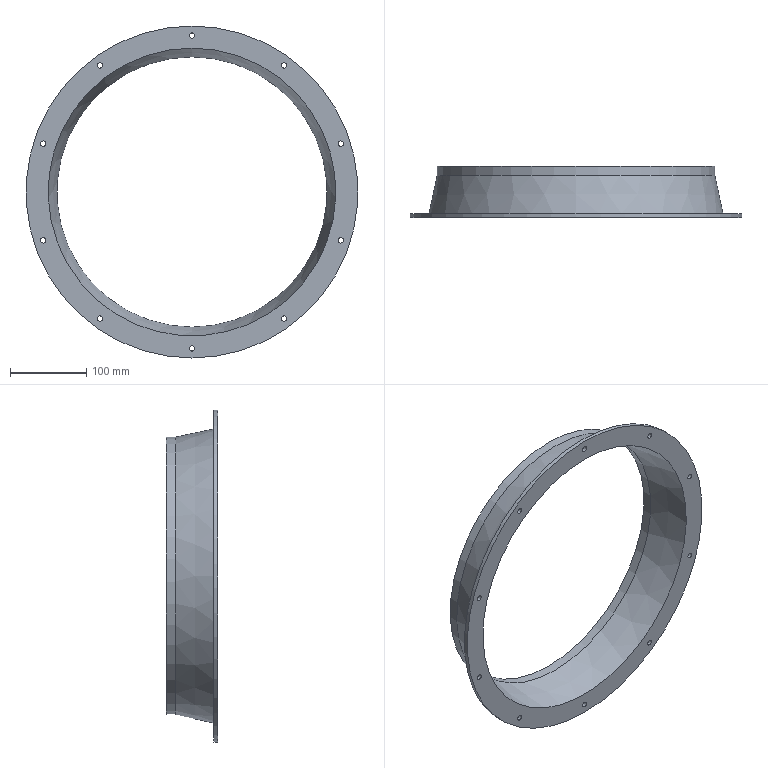Part | STEP file | Upper cover | 1 solid | 18 faces | box 435 x 67 x 435 mm | volume 550559 mm3 | cylinder 13 | plane 3 | cone 2 | commonest cylinder face diameters 7 x10 354 x1 364 x1 435 x1
STEP:
#1=CARTESIAN_POINT('',(0.,67.,182.));
#2=VERTEX_POINT('',#1);
#3=CARTESIAN_POINT('',(0.,67.,0.));
#4=DIRECTION('',(0.,1.,0.));
#5=DIRECTION('',(0.,0.,1.));
#6=AXIS2_PLACEMENT_3D('',#3,#4,#5);
#7=CIRCLE('',#6,182.);
#8=EDGE_CURVE('',#2,#2,#7,.F.);
#9=ORIENTED_EDGE('',*,*,#8,.T.);
#10=EDGE_LOOP('',(#9));
#11=FACE_OUTER_BOUND('',#10,.T.);
#12=CARTESIAN_POINT('',(0.,55.,182.));
#13=VERTEX_POINT('',#12);
#14=CARTESIAN_POINT('',(0.,55.,0.));
#15=DIRECTION('',(0.,1.,0.));
#16=DIRECTION('',(0.,0.,1.));
#17=AXIS2_PLACEMENT_3D('',#14,#15,#16);
#18=CIRCLE('',#17,182.);
#19=EDGE_CURVE('',#13,#13,#18,.T.);
#20=ORIENTED_EDGE('',*,*,#19,.T.);
#21=EDGE_LOOP('',(#20));
#22=FACE_OUTER_BOUND('',#21,.T.);
#23=CARTESIAN_POINT('',(0.,55.,0.));
#24=DIRECTION('',(0.,1.,0.));
#25=DIRECTION('',(0.,0.,1.));
#26=AXIS2_PLACEMENT_3D('',#23,#24,#25);
#27=CYLINDRICAL_SURFACE('',#26,182.);
#28=ADVANCED_FACE('',(#11,#22),#27,.T.);
#29=CARTESIAN_POINT('',(0.,67.,177.));
#30=VERTEX_POINT('',#29);
#31=CARTESIAN_POINT('',(0.,67.,0.));
#32=DIRECTION('',(0.,1.,0.));
#33=DIRECTION('',(0.,0.,1.));
#34=AXIS2_PLACEMENT_3D('',#31,#32,#33);
#35=CIRCLE('',#34,177.);
#36=EDGE_CURVE('',#30,#30,#35,.T.);
#37=ORIENTED_EDGE('',*,*,#36,.T.);
#38=EDGE_LOOP('',(#37));
#39=FACE_OUTER_BOUND('',#38,.T.);
#40=CARTESIAN_POINT('',(0.,54.481,177.));
#41=VERTEX_POINT('',#40);
#42=CARTESIAN_POINT('',(0.,54.481,0.));
#43=DIRECTION('',(0.,1.,0.));
#44=DIRECTION('',(0.,0.,1.));
#45=AXIS2_PLACEMENT_3D('',#42,#43,#44);
#46=CIRCLE('',#45,177.);
#47=EDGE_CURVE('',#41,#41,#46,.T.);
#48=ORIENTED_EDGE('',*,*,#47,.F.);
#49=EDGE_LOOP('',(#48));
#50=FACE_OUTER_BOUND('',#49,.T.);
#51=CARTESIAN_POINT('',(0.,85.,0.));
#52=DIRECTION('',(0.,1.,0.));
#53=DIRECTION('',(0.,0.,1.));
#54=AXIS2_PLACEMENT_3D('',#51,#52,#53);
#55=CYLINDRICAL_SURFACE('',#54,177.);
#56=ADVANCED_FACE('',(#39,#50),#55,.F.);
#57=ORIENTED_EDGE('',*,*,#8,.F.);
#58=EDGE_LOOP('',(#57));
#59=FACE_BOUND('',#58,.T.);
#60=ORIENTED_EDGE('',*,*,#36,.F.);
#61=EDGE_LOOP('',(#60));
#62=FACE_BOUND('',#61,.T.);
#63=CARTESIAN_POINT('',(0.,67.,182.));
#64=DIRECTION('',(0.,1.,0.));
#65=DIRECTION('',(1.,0.,0.));
#66=AXIS2_PLACEMENT_3D('',#63,#64,#65);
#67=PLANE('',#66);
#68=ADVANCED_FACE('',(#59,#62),#67,.T.);
#69=ORIENTED_EDGE('',*,*,#19,.F.);
#70=EDGE_LOOP('',(#69));
#71=FACE_OUTER_BOUND('',#70,.T.);
#72=CARTESIAN_POINT('',(0.,5.,192.5));
#73=VERTEX_POINT('',#72);
#74=CARTESIAN_POINT('',(0.,5.,0.));
#75=DIRECTION('',(0.,1.,0.));
#76=DIRECTION('',(0.,0.,1.));
#77=AXIS2_PLACEMENT_3D('',#74,#75,#76);
#78=CIRCLE('',#77,192.5);
#79=EDGE_CURVE('',#73,#73,#78,.T.);
#80=ORIENTED_EDGE('',*,*,#79,.T.);
#81=EDGE_LOOP('',(#80));
#82=FACE_OUTER_BOUND('',#81,.T.);
#83=CARTESIAN_POINT('',(0.,30.,0.));
#84=DIRECTION('',(0.,-1.,0.));
#85=DIRECTION('',(0.,0.,-1.));
#86=AXIS2_PLACEMENT_3D('',#83,#84,#85);
#87=CONICAL_SURFACE('',#86,187.25,0.207);
#88=ADVANCED_FACE('',(#71,#82),#87,.T.);
#89=ORIENTED_EDGE('',*,*,#47,.T.);
#90=EDGE_LOOP('',(#89));
#91=FACE_OUTER_BOUND('',#90,.T.);
#92=CARTESIAN_POINT('',(0.,0.,188.441));
#93=VERTEX_POINT('',#92);
#94=CARTESIAN_POINT('',(0.,0.,0.));
#95=DIRECTION('',(0.,1.,0.));
#96=DIRECTION('',(0.,0.,1.));
#97=AXIS2_PLACEMENT_3D('',#94,#95,#96);
#98=CIRCLE('',#97,188.441);
#99=EDGE_CURVE('',#93,#93,#98,.T.);
#100=ORIENTED_EDGE('',*,*,#99,.F.);
#101=EDGE_LOOP('',(#100));
#102=FACE_OUTER_BOUND('',#101,.T.);
#103=CARTESIAN_POINT('',(0.,27.24,0.));
#104=DIRECTION('',(0.,-1.,0.));
#105=DIRECTION('',(0.,0.,-1.));
#106=AXIS2_PLACEMENT_3D('',#103,#104,#105);
#107=CONICAL_SURFACE('',#106,182.72,0.207);
#108=ADVANCED_FACE('',(#91,#102),#107,.F.);
#109=CARTESIAN_POINT('',(0.,5.,217.5));
#110=VERTEX_POINT('',#109);
#111=CARTESIAN_POINT('',(0.,5.,0.));
#112=DIRECTION('',(0.,1.,0.));
#113=DIRECTION('',(0.,0.,1.));
#114=AXIS2_PLACEMENT_3D('',#111,#112,#113);
#115=CIRCLE('',#114,217.5);
#116=EDGE_CURVE('',#110,#110,#115,.T.);
#117=ORIENTED_EDGE('',*,*,#116,.T.);
#118=EDGE_LOOP('',(#117));
#119=FACE_BOUND('',#118,.T.);
#120=CARTESIAN_POINT('',(123.328,5.,163.791));
#121=VERTEX_POINT('',#120);
#122=CARTESIAN_POINT('',(120.496,5.,165.848));
#123=DIRECTION('',(0.,1.,0.));
#124=DIRECTION('',(0.809,0.,-0.5878));
#125=AXIS2_PLACEMENT_3D('',#122,#123,#124);
#126=CIRCLE('',#125,3.5);
#127=EDGE_CURVE('',#121,#121,#126,.F.);
#128=ORIENTED_EDGE('',*,*,#127,.T.);
#129=EDGE_LOOP('',(#128));
#130=FACE_BOUND('',#129,.T.);
#131=CARTESIAN_POINT('',(196.048,5.,60.02));
#132=VERTEX_POINT('',#131);
#133=CARTESIAN_POINT('',(194.967,5.,63.348));
#134=DIRECTION('',(0.,1.,0.));
#135=DIRECTION('',(0.309,0.,-0.9511));
#136=AXIS2_PLACEMENT_3D('',#133,#134,#135);
#137=CIRCLE('',#136,3.5);
#138=EDGE_CURVE('',#132,#132,#137,.F.);
#139=ORIENTED_EDGE('',*,*,#138,.T.);
#140=EDGE_LOOP('',(#139));
#141=FACE_BOUND('',#140,.T.);
#142=CARTESIAN_POINT('',(193.885,5.,-66.677));
#143=VERTEX_POINT('',#142);
#144=CARTESIAN_POINT('',(194.967,5.,-63.348));
#145=DIRECTION('',(0.,1.,0.));
#146=DIRECTION('',(-0.309,0.,-0.9511));
#147=AXIS2_PLACEMENT_3D('',#144,#145,#146);
#148=CIRCLE('',#147,3.5);
#149=EDGE_CURVE('',#143,#143,#148,.F.);
#150=ORIENTED_EDGE('',*,*,#149,.T.);
#151=EDGE_LOOP('',(#150));
#152=FACE_BOUND('',#151,.T.);
#153=CARTESIAN_POINT('',(117.664,5.,-167.906));
#154=VERTEX_POINT('',#153);
#155=CARTESIAN_POINT('',(120.496,5.,-165.848));
#156=DIRECTION('',(0.,1.,0.));
#157=DIRECTION('',(-0.809,0.,-0.5878));
#158=AXIS2_PLACEMENT_3D('',#155,#156,#157);
#159=CIRCLE('',#158,3.5);
#160=EDGE_CURVE('',#154,#154,#159,.F.);
#161=ORIENTED_EDGE('',*,*,#160,.T.);
#162=EDGE_LOOP('',(#161));
#163=FACE_BOUND('',#162,.T.);
#164=CARTESIAN_POINT('',(-3.5,5.,-205.));
#165=VERTEX_POINT('',#164);
#166=CARTESIAN_POINT('',(0.,5.,-205.));
#167=DIRECTION('',(0.,1.,0.));
#168=DIRECTION('',(-1.,0.,0.));
#169=AXIS2_PLACEMENT_3D('',#166,#167,#168);
#170=CIRCLE('',#169,3.5);
#171=EDGE_CURVE('',#165,#165,#170,.F.);
#172=ORIENTED_EDGE('',*,*,#171,.T.);
#173=EDGE_LOOP('',(#172));
#174=FACE_BOUND('',#173,.T.);
#175=CARTESIAN_POINT('',(-123.328,5.,-163.791));
#176=VERTEX_POINT('',#175);
#177=CARTESIAN_POINT('',(-120.496,5.,-165.848));
#178=DIRECTION('',(0.,1.,0.));
#179=DIRECTION('',(-0.809,0.,0.5878));
#180=AXIS2_PLACEMENT_3D('',#177,#178,#179);
#181=CIRCLE('',#180,3.5);
#182=EDGE_CURVE('',#176,#176,#181,.F.);
#183=ORIENTED_EDGE('',*,*,#182,.T.);
#184=EDGE_LOOP('',(#183));
#185=FACE_BOUND('',#184,.T.);
#186=CARTESIAN_POINT('',(-196.048,5.,-60.02));
#187=VERTEX_POINT('',#186);
#188=CARTESIAN_POINT('',(-194.967,5.,-63.348));
#189=DIRECTION('',(0.,1.,0.));
#190=DIRECTION('',(-0.309,0.,0.9511));
#191=AXIS2_PLACEMENT_3D('',#188,#189,#190);
#192=CIRCLE('',#191,3.5);
#193=EDGE_CURVE('',#187,#187,#192,.F.);
#194=ORIENTED_EDGE('',*,*,#193,.T.);
#195=EDGE_LOOP('',(#194));
#196=FACE_BOUND('',#195,.T.);
#197=CARTESIAN_POINT('',(-193.885,5.,66.677));
#198=VERTEX_POINT('',#197);
#199=CARTESIAN_POINT('',(-194.967,5.,63.348));
#200=DIRECTION('',(0.,1.,0.));
#201=DIRECTION('',(0.309,0.,0.9511));
#202=AXIS2_PLACEMENT_3D('',#199,#200,#201);
#203=CIRCLE('',#202,3.5);
#204=EDGE_CURVE('',#198,#198,#203,.F.);
#205=ORIENTED_EDGE('',*,*,#204,.T.);
#206=EDGE_LOOP('',(#205));
#207=FACE_BOUND('',#206,.T.);
#208=CARTESIAN_POINT('',(-117.664,5.,167.906));
#209=VERTEX_POINT('',#208);
#210=CARTESIAN_POINT('',(-120.496,5.,165.848));
#211=DIRECTION('',(0.,1.,0.));
#212=DIRECTION('',(0.809,0.,0.5878));
#213=AXIS2_PLACEMENT_3D('',#210,#211,#212);
#214=CIRCLE('',#213,3.5);
#215=EDGE_CURVE('',#209,#209,#214,.F.);
#216=ORIENTED_EDGE('',*,*,#215,.T.);
#217=EDGE_LOOP('',(#216));
#218=FACE_BOUND('',#217,.T.);
#219=ORIENTED_EDGE('',*,*,#79,.F.);
#220=EDGE_LOOP('',(#219));
#221=FACE_BOUND('',#220,.T.);
#222=CARTESIAN_POINT('',(3.5,5.,205.));
#223=VERTEX_POINT('',#222);
#224=CARTESIAN_POINT('',(0.,5.,205.));
#225=DIRECTION('',(0.,1.,0.));
#226=DIRECTION('',(1.,0.,0.));
#227=AXIS2_PLACEMENT_3D('',#224,#225,#226);
#228=CIRCLE('',#227,3.5);
#229=EDGE_CURVE('',#223,#223,#228,.F.);
#230=ORIENTED_EDGE('',*,*,#229,.T.);
#231=EDGE_LOOP('',(#230));
#232=FACE_BOUND('',#231,.T.);
#233=CARTESIAN_POINT('',(0.,5.,0.));
#234=DIRECTION('',(0.,1.,0.));
#235=DIRECTION('',(0.,0.,1.));
#236=AXIS2_PLACEMENT_3D('',#233,#234,#235);
#237=PLANE('',#236);
#238=ADVANCED_FACE('',(#119,#130,#141,#152,#163,#174,#185,#196,#207,#218,#221,#232),#237,.T.);
#239=CARTESIAN_POINT('',(0.,0.,217.5));
#240=VERTEX_POINT('',#239);
#241=CARTESIAN_POINT('',(0.,0.,0.));
#242=DIRECTION('',(0.,1.,0.));
#243=DIRECTION('',(0.,0.,1.));
#244=AXIS2_PLACEMENT_3D('',#241,#242,#243);
#245=CIRCLE('',#244,217.5);
#246=EDGE_CURVE('',#240,#240,#245,.T.);
#247=ORIENTED_EDGE('',*,*,#246,.F.);
#248=EDGE_LOOP('',(#247));
#249=FACE_BOUND('',#248,.T.);
#250=CARTESIAN_POINT('',(123.328,0.,163.791));
#251=VERTEX_POINT('',#250);
#252=CARTESIAN_POINT('',(120.496,0.,165.848));
#253=DIRECTION('',(0.,1.,0.));
#254=DIRECTION('',(0.809,0.,-0.5878));
#255=AXIS2_PLACEMENT_3D('',#252,#253,#254);
#256=CIRCLE('',#255,3.5);
#257=EDGE_CURVE('',#251,#251,#256,.T.);
#258=ORIENTED_EDGE('',*,*,#257,.T.);
#259=EDGE_LOOP('',(#258));
#260=FACE_BOUND('',#259,.T.);
#261=CARTESIAN_POINT('',(196.048,0.,60.02));
#262=VERTEX_POINT('',#261);
#263=CARTESIAN_POINT('',(194.967,0.,63.348));
#264=DIRECTION('',(0.,1.,0.));
#265=DIRECTION('',(0.309,0.,-0.9511));
#266=AXIS2_PLACEMENT_3D('',#263,#264,#265);
#267=CIRCLE('',#266,3.5);
#268=EDGE_CURVE('',#262,#262,#267,.T.);
#269=ORIENTED_EDGE('',*,*,#268,.T.);
#270=EDGE_LOOP('',(#269));
#271=FACE_BOUND('',#270,.T.);
#272=CARTESIAN_POINT('',(193.885,0.,-66.677));
#273=VERTEX_POINT('',#272);
#274=CARTESIAN_POINT('',(194.967,0.,-63.348));
#275=DIRECTION('',(0.,1.,0.));
#276=DIRECTION('',(-0.309,0.,-0.9511));
#277=AXIS2_PLACEMENT_3D('',#274,#275,#276);
#278=CIRCLE('',#277,3.5);
#279=EDGE_CURVE('',#273,#273,#278,.T.);
#280=ORIENTED_EDGE('',*,*,#279,.T.);
#281=EDGE_LOOP('',(#280));
#282=FACE_BOUND('',#281,.T.);
#283=CARTESIAN_POINT('',(117.664,0.,-167.906));
#284=VERTEX_POINT('',#283);
#285=CARTESIAN_POINT('',(120.496,0.,-165.848));
#286=DIRECTION('',(0.,1.,0.));
#287=DIRECTION('',(-0.809,0.,-0.5878));
#288=AXIS2_PLACEMENT_3D('',#285,#286,#287);
#289=CIRCLE('',#288,3.5);
#290=EDGE_CURVE('',#284,#284,#289,.T.);
#291=ORIENTED_EDGE('',*,*,#290,.T.);
#292=EDGE_LOOP('',(#291));
#293=FACE_BOUND('',#292,.T.);
#294=CARTESIAN_POINT('',(-3.5,0.,-205.));
#295=VERTEX_POINT('',#294);
#296=CARTESIAN_POINT('',(0.,0.,-205.));
#297=DIRECTION('',(0.,1.,0.));
#298=DIRECTION('',(-1.,0.,0.));
#299=AXIS2_PLACEMENT_3D('',#296,#297,#298);
#300=CIRCLE('',#299,3.5);
#301=EDGE_CURVE('',#295,#295,#300,.T.);
#302=ORIENTED_EDGE('',*,*,#301,.T.);
#303=EDGE_LOOP('',(#302));
#304=FACE_BOUND('',#303,.T.);
#305=CARTESIAN_POINT('',(-123.328,0.,-163.791));
#306=VERTEX_POINT('',#305);
#307=CARTESIAN_POINT('',(-120.496,0.,-165.848));
#308=DIRECTION('',(0.,1.,0.));
#309=DIRECTION('',(-0.809,0.,0.5878));
#310=AXIS2_PLACEMENT_3D('',#307,#308,#309);
#311=CIRCLE('',#310,3.5);
#312=EDGE_CURVE('',#306,#306,#311,.T.);
#313=ORIENTED_EDGE('',*,*,#312,.T.);
#314=EDGE_LOOP('',(#313));
#315=FACE_BOUND('',#314,.T.);
#316=CARTESIAN_POINT('',(-196.048,0.,-60.02));
#317=VERTEX_POINT('',#316);
#318=CARTESIAN_POINT('',(-194.967,0.,-63.348));
#319=DIRECTION('',(0.,1.,0.));
#320=DIRECTION('',(-0.309,0.,0.9511));
#321=AXIS2_PLACEMENT_3D('',#318,#319,#320);
#322=CIRCLE('',#321,3.5);
#323=EDGE_CURVE('',#317,#317,#322,.T.);
#324=ORIENTED_EDGE('',*,*,#323,.T.);
#325=EDGE_LOOP('',(#324));
#326=FACE_BOUND('',#325,.T.);
#327=CARTESIAN_POINT('',(-193.885,0.,66.677));
#328=VERTEX_POINT('',#327);
#329=CARTESIAN_POINT('',(-194.967,0.,63.348));
#330=DIRECTION('',(0.,1.,0.));
#331=DIRECTION('',(0.309,0.,0.9511));
#332=AXIS2_PLACEMENT_3D('',#329,#330,#331);
#333=CIRCLE('',#332,3.5);
#334=EDGE_CURVE('',#328,#328,#333,.T.);
#335=ORIENTED_EDGE('',*,*,#334,.T.);
#336=EDGE_LOOP('',(#335));
#337=FACE_BOUND('',#336,.T.);
#338=CARTESIAN_POINT('',(-117.664,0.,167.906));
#339=VERTEX_POINT('',#338);
#340=CARTESIAN_POINT('',(-120.496,0.,165.848));
#341=DIRECTION('',(0.,1.,0.));
#342=DIRECTION('',(0.809,0.,0.5878));
#343=AXIS2_PLACEMENT_3D('',#340,#341,#342);
#344=CIRCLE('',#343,3.5);
#345=EDGE_CURVE('',#339,#339,#344,.T.);
#346=ORIENTED_EDGE('',*,*,#345,.T.);
#347=EDGE_LOOP('',(#346));
#348=FACE_BOUND('',#347,.T.);
#349=ORIENTED_EDGE('',*,*,#99,.T.);
#350=EDGE_LOOP('',(#349));
#351=FACE_BOUND('',#350,.T.);
#352=CARTESIAN_POINT('',(3.5,0.,205.));
#353=VERTEX_POINT('',#352);
#354=CARTESIAN_POINT('',(0.,0.,205.));
#355=DIRECTION('',(0.,1.,0.));
#356=DIRECTION('',(1.,0.,0.));
#357=AXIS2_PLACEMENT_3D('',#354,#355,#356);
#358=CIRCLE('',#357,3.5);
#359=EDGE_CURVE('',#353,#353,#358,.T.);
#360=ORIENTED_EDGE('',*,*,#359,.T.);
#361=EDGE_LOOP('',(#360));
#362=FACE_BOUND('',#361,.T.);
#363=CARTESIAN_POINT('',(0.,0.,0.));
#364=DIRECTION('',(0.,-1.,0.));
#365=DIRECTION('',(0.,0.,1.));
#366=AXIS2_PLACEMENT_3D('',#363,#364,#365);
#367=PLANE('',#366);
#368=ADVANCED_FACE('',(#249,#260,#271,#282,#293,#304,#315,#326,#337,#348,#351,#362),#367,.T.);
#369=ORIENTED_EDGE('',*,*,#116,.F.);
#370=EDGE_LOOP('',(#369));
#371=FACE_OUTER_BOUND('',#370,.T.);
#372=ORIENTED_EDGE('',*,*,#246,.T.);
#373=EDGE_LOOP('',(#372));
#374=FACE_OUTER_BOUND('',#373,.T.);
#375=CARTESIAN_POINT('',(0.,0.,0.));
#376=DIRECTION('',(0.,1.,0.));
#377=DIRECTION('',(0.,0.,1.));
#378=AXIS2_PLACEMENT_3D('',#375,#376,#377);
#379=CYLINDRICAL_SURFACE('',#378,217.5);
#380=ADVANCED_FACE('',(#371,#374),#379,.T.);
#381=ORIENTED_EDGE('',*,*,#127,.F.);
#382=EDGE_LOOP('',(#381));
#383=FACE_OUTER_BOUND('',#382,.T.);
#384=ORIENTED_EDGE('',*,*,#257,.F.);
#385=EDGE_LOOP('',(#384));
#386=FACE_OUTER_BOUND('',#385,.T.);
#387=CARTESIAN_POINT('',(120.496,-35.,165.848));
#388=DIRECTION('',(0.,1.,0.));
#389=DIRECTION('',(0.809,0.,-0.5878));
#390=AXIS2_PLACEMENT_3D('',#387,#388,#389);
#391=CYLINDRICAL_SURFACE('',#390,3.5);
#392=ADVANCED_FACE('',(#383,#386),#391,.F.);
#393=ORIENTED_EDGE('',*,*,#138,.F.);
#394=EDGE_LOOP('',(#393));
#395=FACE_OUTER_BOUND('',#394,.T.);
#396=ORIENTED_EDGE('',*,*,#268,.F.);
#397=EDGE_LOOP('',(#396));
#398=FACE_OUTER_BOUND('',#397,.T.);
#399=CARTESIAN_POINT('',(194.967,-35.,63.348));
#400=DIRECTION('',(0.,1.,0.));
#401=DIRECTION('',(0.309,0.,-0.9511));
#402=AXIS2_PLACEMENT_3D('',#399,#400,#401);
#403=CYLINDRICAL_SURFACE('',#402,3.5);
#404=ADVANCED_FACE('',(#395,#398),#403,.F.);
#405=ORIENTED_EDGE('',*,*,#149,.F.);
#406=EDGE_LOOP('',(#405));
#407=FACE_OUTER_BOUND('',#406,.T.);
#408=ORIENTED_EDGE('',*,*,#279,.F.);
#409=EDGE_LOOP('',(#408));
#410=FACE_OUTER_BOUND('',#409,.T.);
#411=CARTESIAN_POINT('',(194.967,-35.,-63.348));
#412=DIRECTION('',(0.,1.,0.));
#413=DIRECTION('',(-0.309,0.,-0.9511));
#414=AXIS2_PLACEMENT_3D('',#411,#412,#413);
#415=CYLINDRICAL_SURFACE('',#414,3.5);
#416=ADVANCED_FACE('',(#407,#410),#415,.F.);
#417=ORIENTED_EDGE('',*,*,#160,.F.);
#418=EDGE_LOOP('',(#417));
#419=FACE_OUTER_BOUND('',#418,.T.);
#420=ORIENTED_EDGE('',*,*,#290,.F.);
#421=EDGE_LOOP('',(#420));
#422=FACE_OUTER_BOUND('',#421,.T.);
#423=CARTESIAN_POINT('',(120.496,-35.,-165.848));
#424=DIRECTION('',(0.,1.,0.));
#425=DIRECTION('',(-0.809,0.,-0.5878));
#426=AXIS2_PLACEMENT_3D('',#423,#424,#425);
#427=CYLINDRICAL_SURFACE('',#426,3.5);
#428=ADVANCED_FACE('',(#419,#422),#427,.F.);
#429=ORIENTED_EDGE('',*,*,#171,.F.);
#430=EDGE_LOOP('',(#429));
#431=FACE_OUTER_BOUND('',#430,.T.);
#432=ORIENTED_EDGE('',*,*,#301,.F.);
#433=EDGE_LOOP('',(#432));
#434=FACE_OUTER_BOUND('',#433,.T.);
#435=CARTESIAN_POINT('',(0.,-35.,-205.));
#436=DIRECTION('',(0.,1.,0.));
#437=DIRECTION('',(-1.,0.,0.));
#438=AXIS2_PLACEMENT_3D('',#435,#436,#437);
#439=CYLINDRICAL_SURFACE('',#438,3.5);
#440=ADVANCED_FACE('',(#431,#434),#439,.F.);
#441=ORIENTED_EDGE('',*,*,#182,.F.);
#442=EDGE_LOOP('',(#441));
#443=FACE_OUTER_BOUND('',#442,.T.);
#444=ORIENTED_EDGE('',*,*,#312,.F.);
#445=EDGE_LOOP('',(#444));
#446=FACE_OUTER_BOUND('',#445,.T.);
#447=CARTESIAN_POINT('',(-120.496,-35.,-165.848));
#448=DIRECTION('',(0.,1.,0.));
#449=DIRECTION('',(-0.809,0.,0.5878));
#450=AXIS2_PLACEMENT_3D('',#447,#448,#449);
#451=CYLINDRICAL_SURFACE('',#450,3.5);
#452=ADVANCED_FACE('',(#443,#446),#451,.F.);
#453=ORIENTED_EDGE('',*,*,#193,.F.);
#454=EDGE_LOOP('',(#453));
#455=FACE_OUTER_BOUND('',#454,.T.);
#456=ORIENTED_EDGE('',*,*,#323,.F.);
#457=EDGE_LOOP('',(#456));
#458=FACE_OUTER_BOUND('',#457,.T.);
#459=CARTESIAN_POINT('',(-194.967,-35.,-63.348));
#460=DIRECTION('',(0.,1.,0.));
#461=DIRECTION('',(-0.309,0.,0.9511));
#462=AXIS2_PLACEMENT_3D('',#459,#460,#461);
#463=CYLINDRICAL_SURFACE('',#462,3.5);
#464=ADVANCED_FACE('',(#455,#458),#463,.F.);
#465=ORIENTED_EDGE('',*,*,#204,.F.);
#466=EDGE_LOOP('',(#465));
#467=FACE_OUTER_BOUND('',#466,.T.);
#468=ORIENTED_EDGE('',*,*,#334,.F.);
#469=EDGE_LOOP('',(#468));
#470=FACE_OUTER_BOUND('',#469,.T.);
#471=CARTESIAN_POINT('',(-194.967,-35.,63.348));
#472=DIRECTION('',(0.,1.,0.));
#473=DIRECTION('',(0.309,0.,0.9511));
#474=AXIS2_PLACEMENT_3D('',#471,#472,#473);
#475=CYLINDRICAL_SURFACE('',#474,3.5);
#476=ADVANCED_FACE('',(#467,#470),#475,.F.);
#477=ORIENTED_EDGE('',*,*,#215,.F.);
#478=EDGE_LOOP('',(#477));
#479=FACE_OUTER_BOUND('',#478,.T.);
#480=ORIENTED_EDGE('',*,*,#345,.F.);
#481=EDGE_LOOP('',(#480));
#482=FACE_OUTER_BOUND('',#481,.T.);
#483=CARTESIAN_POINT('',(-120.496,-35.,165.848));
#484=DIRECTION('',(0.,1.,0.));
#485=DIRECTION('',(0.809,0.,0.5878));
#486=AXIS2_PLACEMENT_3D('',#483,#484,#485);
#487=CYLINDRICAL_SURFACE('',#486,3.5);
#488=ADVANCED_FACE('',(#479,#482),#487,.F.);
#489=ORIENTED_EDGE('',*,*,#229,.F.);
#490=EDGE_LOOP('',(#489));
#491=FACE_OUTER_BOUND('',#490,.T.);
#492=ORIENTED_EDGE('',*,*,#359,.F.);
#493=EDGE_LOOP('',(#492));
#494=FACE_OUTER_BOUND('',#493,.T.);
#495=CARTESIAN_POINT('',(0.,-35.,205.));
#496=DIRECTION('',(0.,1.,0.));
#497=DIRECTION('',(1.,0.,0.));
#498=AXIS2_PLACEMENT_3D('',#495,#496,#497);
#499=CYLINDRICAL_SURFACE('',#498,3.5);
#500=ADVANCED_FACE('',(#491,#494),#499,.F.);
#501=CLOSED_SHELL('',(#28,#56,#68,#88,#108,#238,#368,#380,#392,#404,#416,#428,#440,#452,#464,#476,#488,#500));
#502=MANIFOLD_SOLID_BREP('',#501);
#503=(LENGTH_UNIT()NAMED_UNIT(*)SI_UNIT(.MILLI.,.METRE.));
#504=UNCERTAINTY_MEASURE_WITH_UNIT(LENGTH_MEASURE(0.00001),#503,'','');
#505=(NAMED_UNIT(*)PLANE_ANGLE_UNIT()SI_UNIT($,.RADIAN.));
#506=(NAMED_UNIT(*)SI_UNIT($,.STERADIAN.)SOLID_ANGLE_UNIT());
#507=(GEOMETRIC_REPRESENTATION_CONTEXT(3)GLOBAL_UNCERTAINTY_ASSIGNED_CONTEXT((#504))GLOBAL_UNIT_ASSIGNED_CONTEXT((#503,#505,#506))REPRESENTATION_CONTEXT('',''));
#508=ADVANCED_BREP_SHAPE_REPRESENTATION('',(#502),#507);